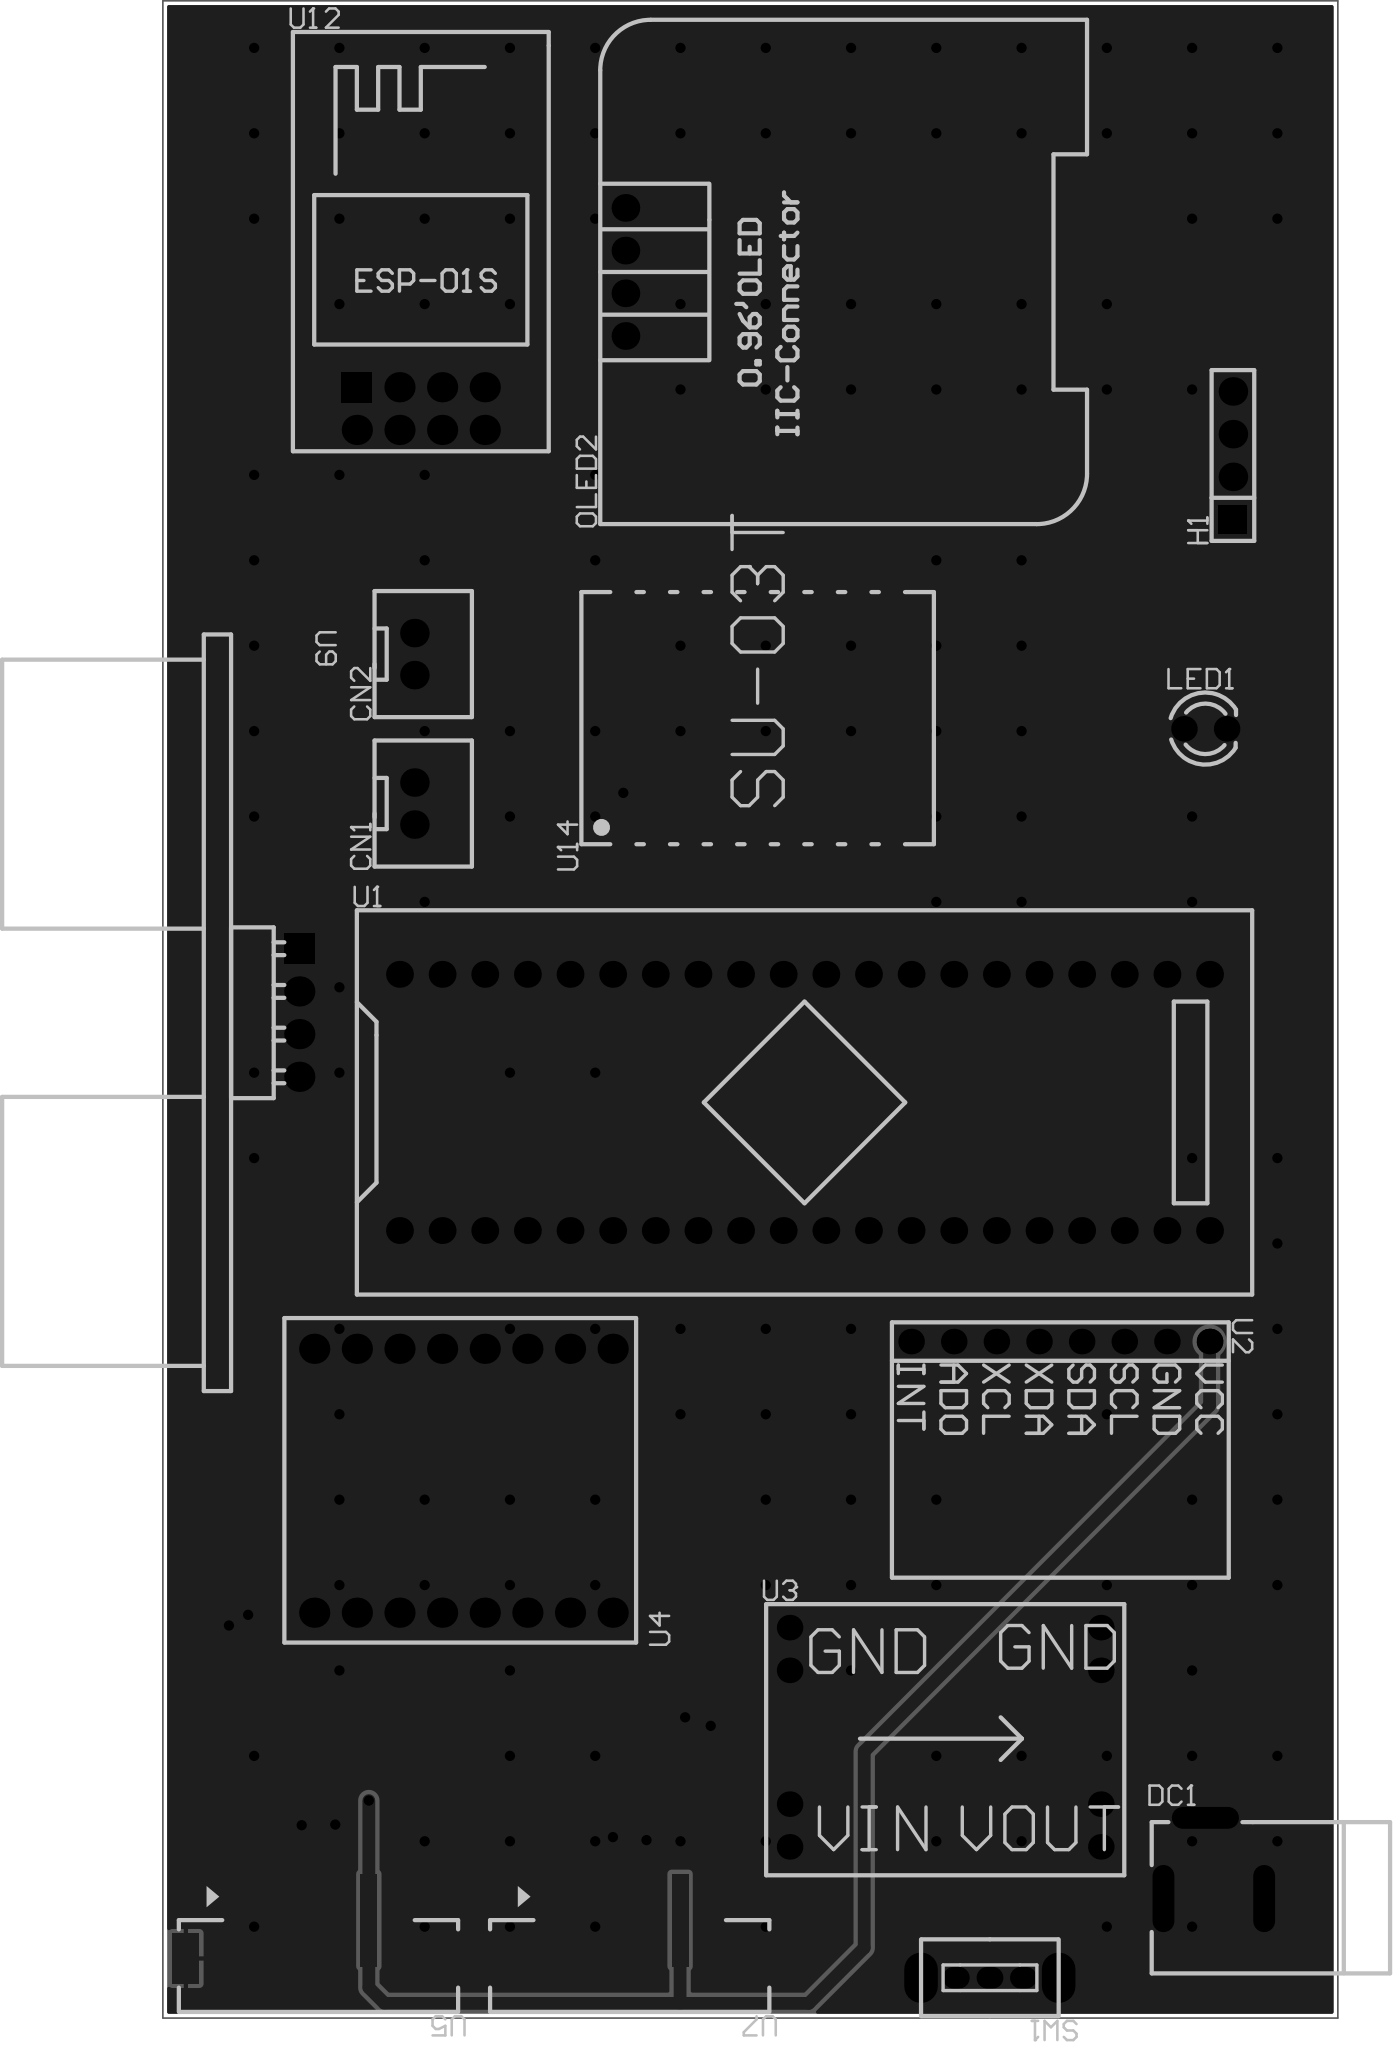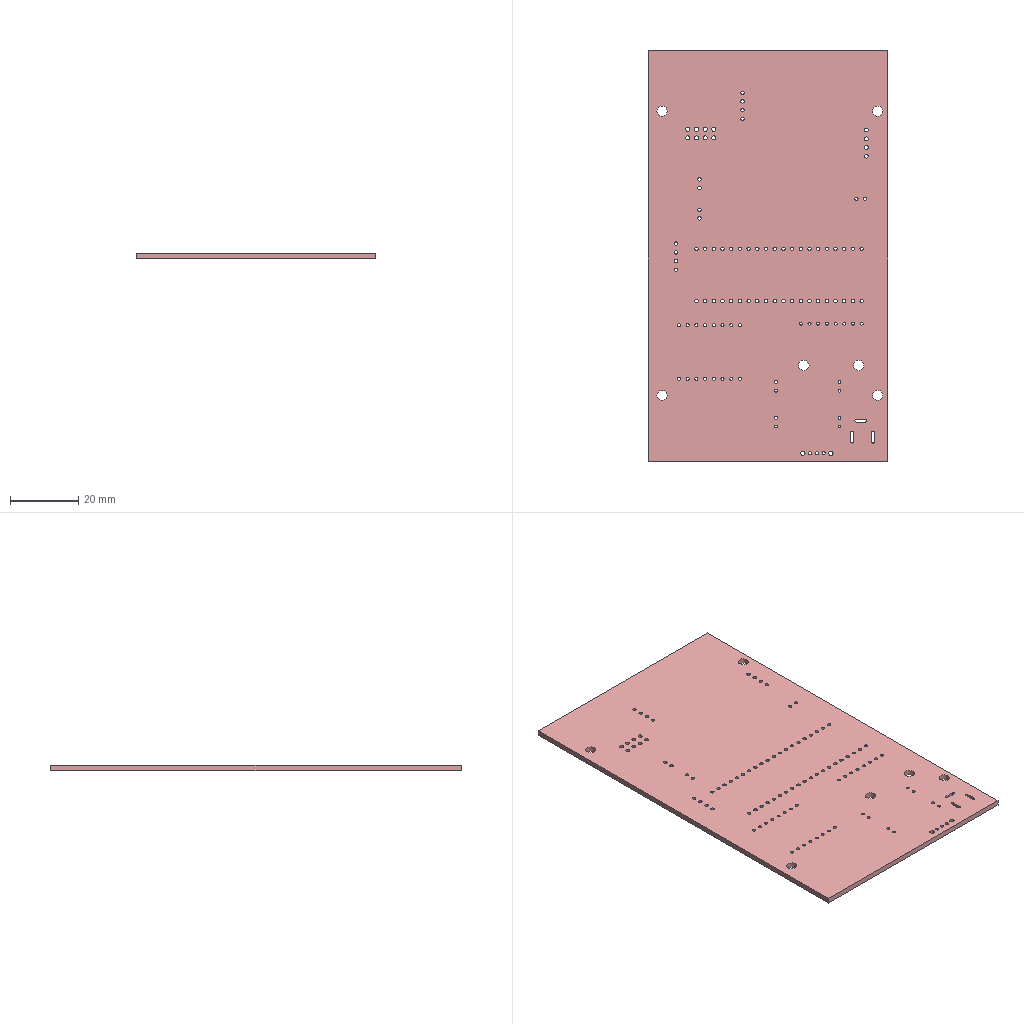Circuit board layout | Altium Designer | box 70 x 120 x 1.6 mm
Layer stack:
# Altium Designer layer stack of  (unit mm; dielectric type: 0 none, 1 core, 2 prepreg, 3 surface material)
index,name,kind,layer,copper_thickness_mm,dielectric_type,dielectric_thickness_mm,dielectric_material,dielectric_constant
0,Top Paste Mask Layer,other,,,,,,
1,Top Silkscreen Layer,other,,,,,,
2,Top Solder Mask Layer,dielectric,,,3,0.01,,3.3
3,Top Layer,copper,Top Layer,0.035,,,,
4,Dielectric1,dielectric,,,3,1.51,FR4,4.5
5,Bottom Layer,copper,Bottom Layer,0.035,,,,
6,Bottom Solder Mask Layer,dielectric,,,3,0.01,,3.3
7,Bottom Silkscreen Layer,other,,,,,,
8,Bottom Paste Mask Layer,other,,,,,,
# drill layer pairs: low layer,high layer
drill_pair,Top Layer,Bottom Layer
Part placement:
Designator,Comment,Layer,Footprint,Center-X(mm),Center-Y(mm),Rotation
LED1,,TopLayer,LED_TH-3mm,478.028,164.973,0
OLED2,,TopLayer,0.96OLED_4P,443.484,192.151,90
U1,STM32F103C8T6-Card,TopLayer,CONN-TH_L53.3-W22.9_STM32F103C8T6-CARD,454.152,142.748,0
U2,MPU6050 module,TopLayer,MPU6050,469.392,128.524,270
U3,,TopLayer,MP1584主控,462.534,104.986,0
U4,,TopLayer,tb6612,433.832,120.244,90
U5,MXPH-2.0-06P-LT1-0-A,TopLayer,CONN-SMD_6P-P2.00_MXPH-2.0-6P-LT1-0-A,425.196,92.964,180
U7,MXPH-2.0-06P-LT1-0-A,TopLayer,CONN-SMD_6P-P2.00_MXPH-2.0-6P-LT1-0-A,443.738,92.964,180
U9,HC-SR04,TopLayer,TH_HC-SR04V,424.053,148.082,270
U12,ESP-01S,TopLayer,WIFIM-TH_ESP-01S,431.292,184.023,0
U14,,TopLayer,SU-03T,451.359,165.608,90
DC1,,TopLayer,DC-2.0,478.536,97.79,0
SW1,,TopLayer,拨动开关,465.193,90.678,180
CN1,XH2.54*2P_through-hole,TopLayer,CONN-TH_2P-P2.50-XH2.54-2P,430.911,160.528,90
CN2,XH2.54*2P_through-hole,TopLayer,CONN-TH_2P-P2.50-XH2.54-2P,430.911,169.418,90
H1,,TopLayer,HDR-TH_4P-P2.54-V-M,479.675,181.232,90
Pad and via stacks:
# Altium Designer via and pad stacks of  (unit mm). Each distinct definition once, with the count of objects using it.
# via: kind,start_layer,end_layer,hole_mm,diameter_mm,mode(0 simple;1 top-mid-bottom;2 full stack),diameter_per_layer,count,example_net
# pad: kind,layer,hole_mm,hole_type(0 round;1 square;2 slot),plating,top_size,top_shape(1 round;2 rect;3 octagon;9 rounded rect),mid_size,bottom_size,mode,footprint,size_per_layer,count,example
pad,Multi-Layer,0.9144,0,plated,1.524x1.524,1,1.524x1.524,1.524x1.524,0,LED_TH-3mm,,2,LED1.1
pad,Multi-Layer,1,0,plated,1.65x1.65,1,1.65x1.65,1.65x1.65,0,0.96OLED_4P,,4,OLED2.4
pad,Multi-Layer,1,0,plated,1.6x1.6,1,1.6x1.6,1.6x1.6,0,CONN-TH_L53.3-W22.9_STM32F103C8T6-CARD,,40,U1.1
pad,Multi-Layer,0.9144,0,plated,1.524x1.524,1,1.524x1.524,1.524x1.524,0,MPU6050,,8,U2.1
pad,Multi-Layer,0.8382,0,plated,1.524x1.524,1,1.524x1.524,1.524x1.524,0,MP1584\u00D6\u00F7\u00BF\u00D8,,8,U3.1
pad,Multi-Layer,0.9,0,plated,1.8x1.8,1,1.8x1.8,1.8x1.8,0,tb6612,,16,U4.1
pad,Multi-Layer,1.001,0,plated,1.8x1.8,1,1.8x1.8,1.8x1.8,0,TH_HC-SR04V,,3,U9.4
pad,Multi-Layer,1.001,0,plated,1.8x1.8,2,1.8x1.8,1.8x1.8,0,TH_HC-SR04V,,1,U9.1
pad,Multi-Layer,1.2,0,plated,1.8x1.8,2,1.8x1.8,1.8x1.8,0,WIFIM-TH_ESP-01S,,1,U12.1
pad,Multi-Layer,1.2,0,plated,1.8x1.8,1,1.8x1.8,1.8x1.8,0,WIFIM-TH_ESP-01S,,7,U12.2
pad,Multi-Layer,0.8001,2,plated,4x1.3,1,4x1.3,4x1.3,0,DC-2.0,,3,DC1.2
pad,Multi-Layer,0.8992,0,plated,1.6x1.3,1,1.6x1.3,1.6x1.3,0,\u00B2\u00A6\u00B6\u00AF\u00BF\u00AA\u00B9\u00D8,,3,SW1.1
pad,Multi-Layer,1.3,0,plated,3x1.999,1,3x1.999,3x1.999,0,\u00B2\u00A6\u00B6\u00AF\u00BF\u00AA\u00B9\u00D8,,2,SW1.4
pad,Multi-Layer,1.05,0,plated,1.7x1.7,1,1.7x1.7,1.7x1.7,0,CONN-TH_2P-P2.50-XH2.54-2P,,4,CN1.2
pad,Multi-Layer,1.1,0,plated,1.7x1.7,2,1.7x1.7,1.7x1.7,0,HDR-TH_4P-P2.54-V-M,,1,H1.1
pad,Multi-Layer,1.1,0,plated,1.7x1.7,1,1.7x1.7,1.7x1.7,0,HDR-TH_4P-P2.54-V-M,,3,H1.2
pad,Top Layer,0,0,plated,1x5.5,2,1x5.5,1x5.5,0,CONN-SMD_6P-P2.00_MXPH-2.0-6P-LT1-0-A,,12,U5.1
pad,Top Layer,0,0,plated,1.6x3,2,1.6x3,1.6x3,0,CONN-SMD_6P-P2.00_MXPH-2.0-6P-LT1-0-A,,4,U5.8
pad,Top Layer,0,0,plated,3x1,2,3x1,3x1,0,SU-03T,,18,U14.1
via,Top Layer,Bottom Layer,0.3048,0.61,0,,162,PA1
Copper pours:
name,layer,net,type(0 solid;1 hatched;2 none)
Bottom Layer-GND,Bottom Layer,GND,0
Bottom Layer-GND 1,Bottom Layer,GND,0
Top Layer-GND,Top Layer,GND,0
Top Layer-GND 1,Top Layer,GND,0
Design rules, without the lines most boards share:
# Altium Designer design rules of  (exported by Altium Designer, unit mm)
# columns: name | kind | enabled | priority | scope1 | scope2 | descriptor | typed fields (field=value)
Copper_copperRegion_copperThickness1oz | 0 | disabled | 4 | All | All | Clearance Constraint (Gap=5.984mil) (Disabled)(All),(All) | gap=0.152
Copper_copperRegion_copperThickness1oz_1 | 63 | disabled | 4 | All | All | Board Clearance Constraint (Gap=0mil) (Disabled)(All) |
Copper_copperRegion_Copper_copperRegion | 0 | disabled | 5 | All | All | Clearance Constraint (Gap=5.984mil) (Disabled)(All),(All) | gap=0.152
Copper_copperRegion_Copper_copperRegion_1 | 63 | disabled | 5 | All | All | Board Clearance Constraint (Gap=0mil) (Disabled)(All) |
copperThickness1oz | 0 | enabled | 6 | All | All | Clearance Constraint (Gap=5.984mil) (All),(All) | gap=0.152
copperThickness1oz_1 | 63 | enabled | 6 | All | All | Board Clearance Constraint (Gap=0mil) (All) |
copperRegion_copperThickness1oz | 20 | disabled | 1 | All | All | Polygon Connect Rule(Relief Connect )(Conductor Width=10mil) (Relief Angle=90 Angle) (Entries=4) (Air Gap Width=10mil) (Disabled)(All),(All) | connect_style(0=relief,1=direct,2=none)=0 relief_conductor_width=0.254 relief_entries=4
copperRegion_Copper_copperRegion | 20 | disabled | 2 | All | All | Polygon Connect Rule(Relief Connect )(Conductor Width=10mil) (Relief Angle=90 Angle) (Entries=4) (Air Gap Width=10mil) (Disabled)(All),(All) | connect_style(0=relief,1=direct,2=none)=0 relief_conductor_width=0.254 relief_entries=4
copperRegion | 20 | enabled | 3 | All | All | Polygon Connect Rule(Relief Connect )(Conductor Width=10mil) (Relief Angle=90 Angle) (Entries=4) (Air Gap Width=10mil) (All),(All) | connect_style(0=relief,1=direct,2=none)=0 relief_conductor_width=0.254 relief_entries=4